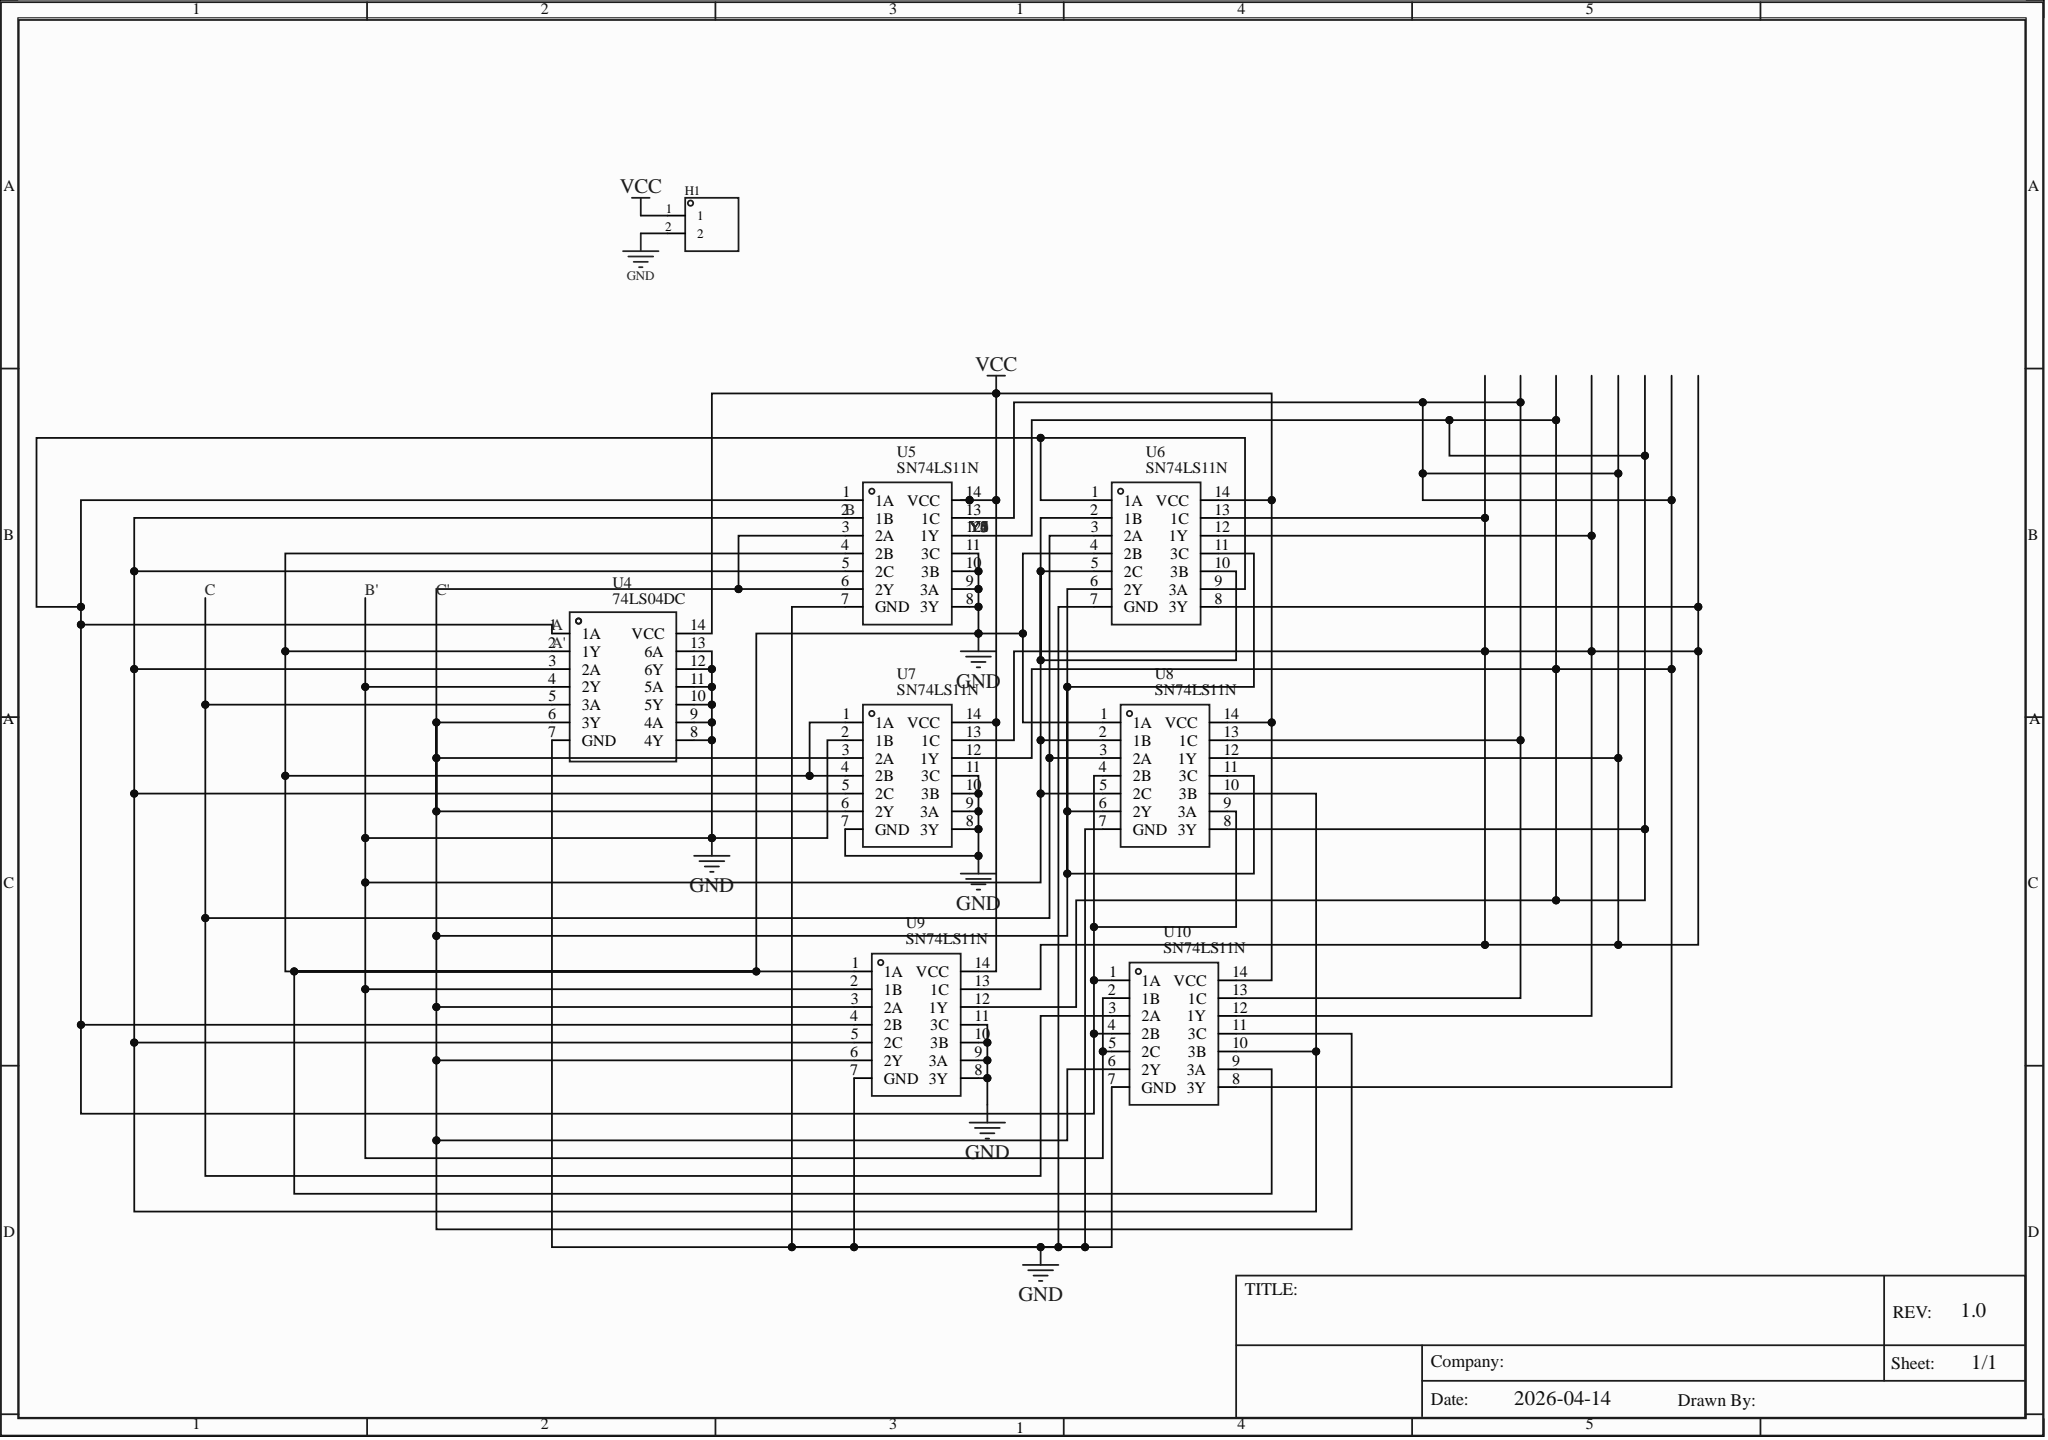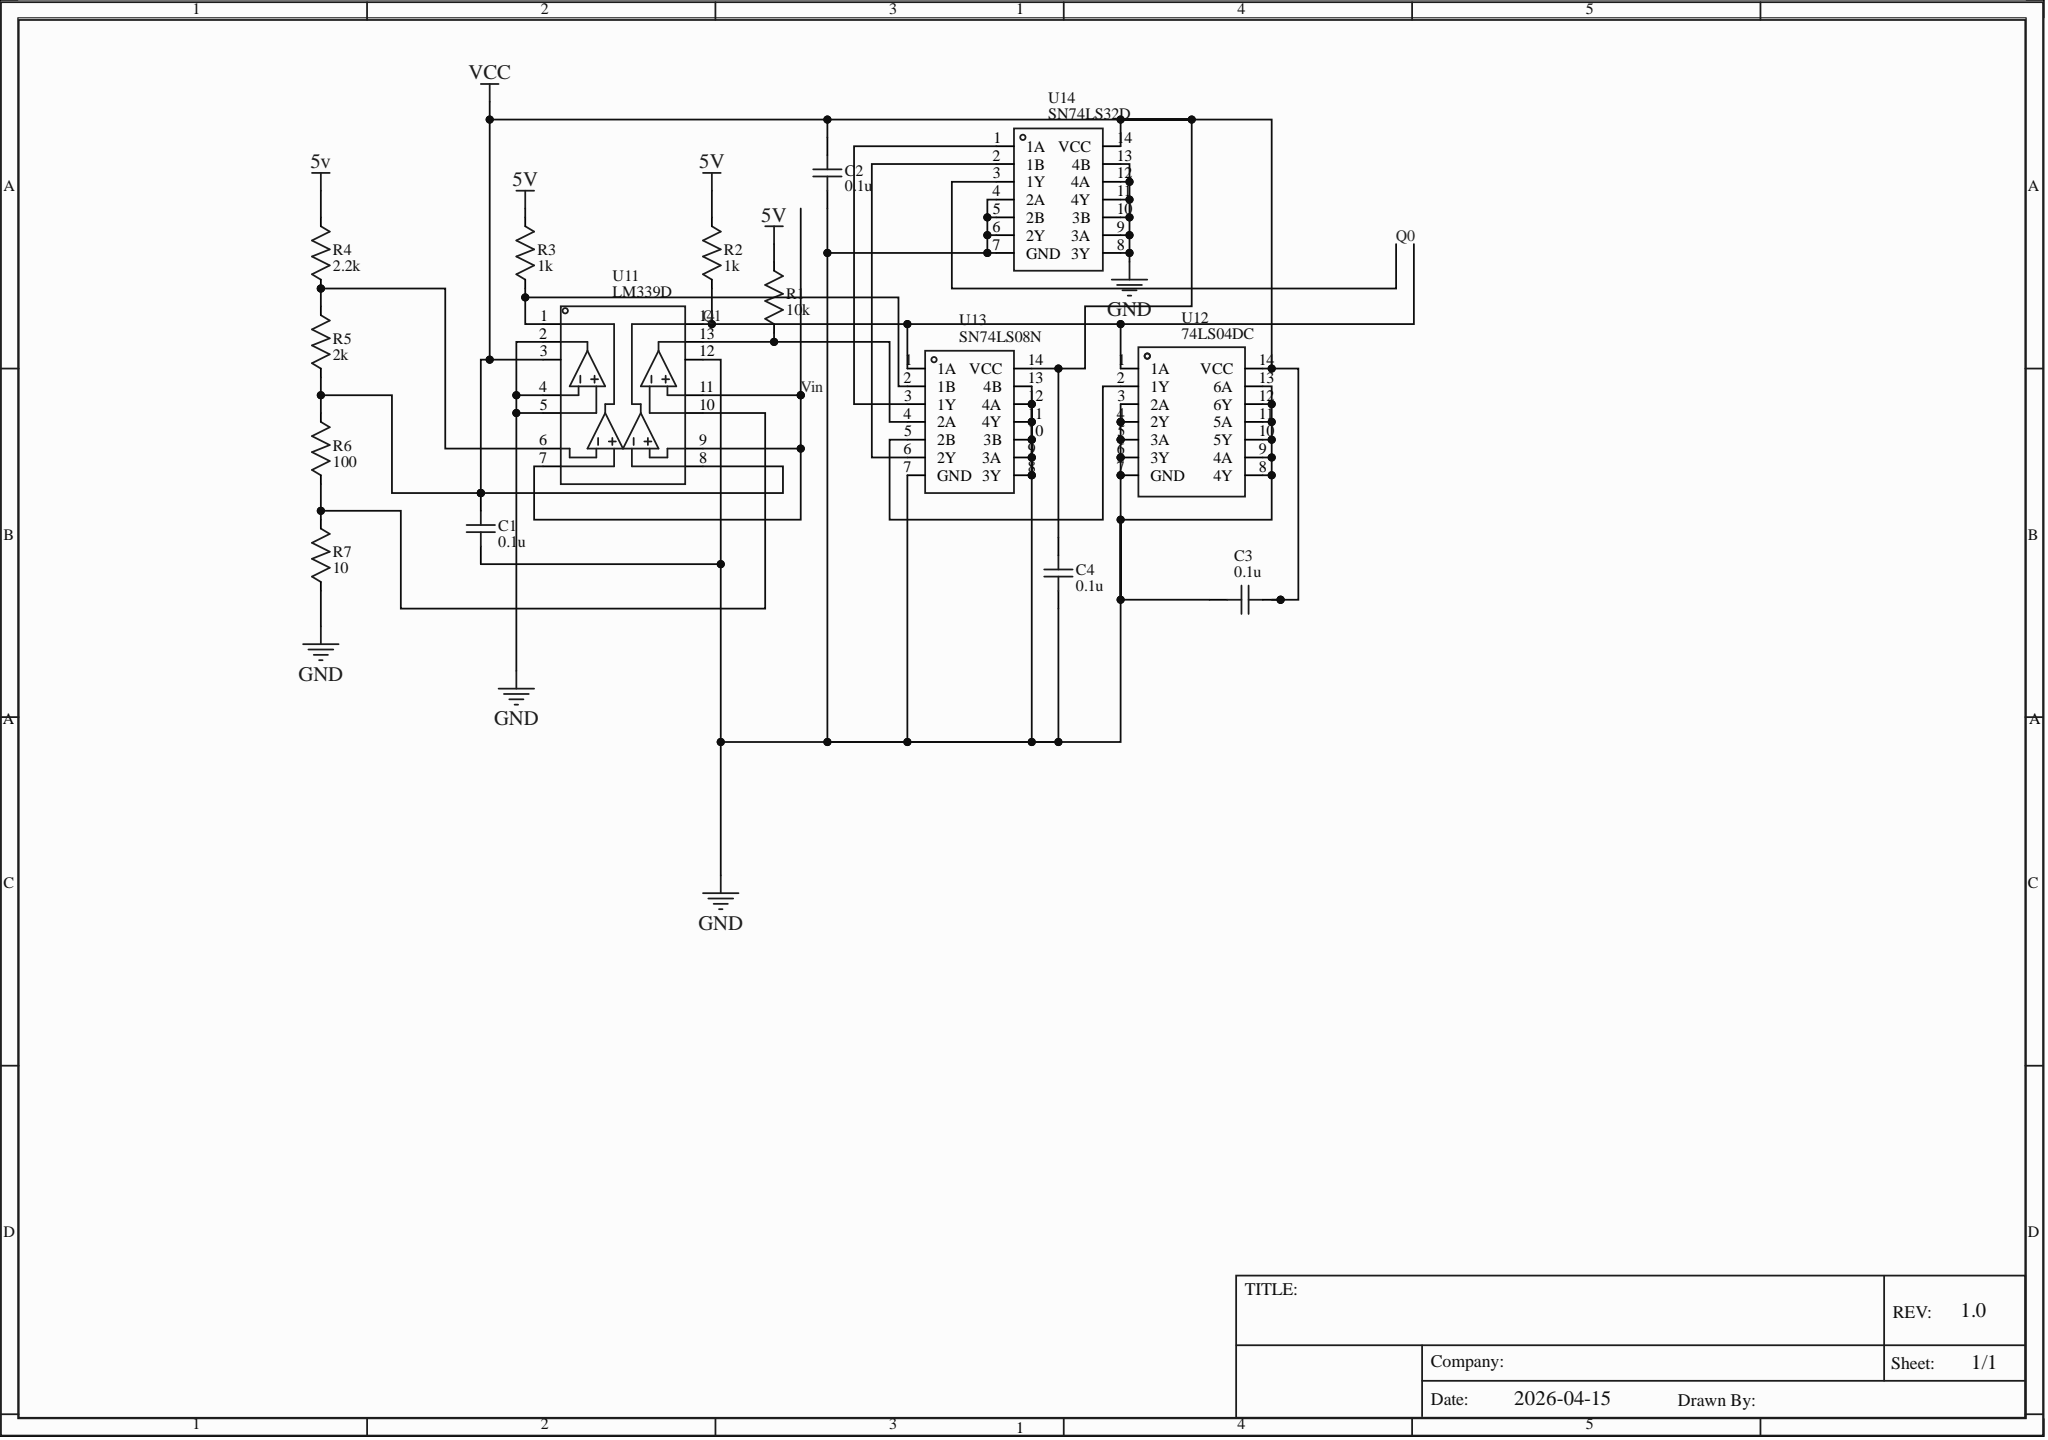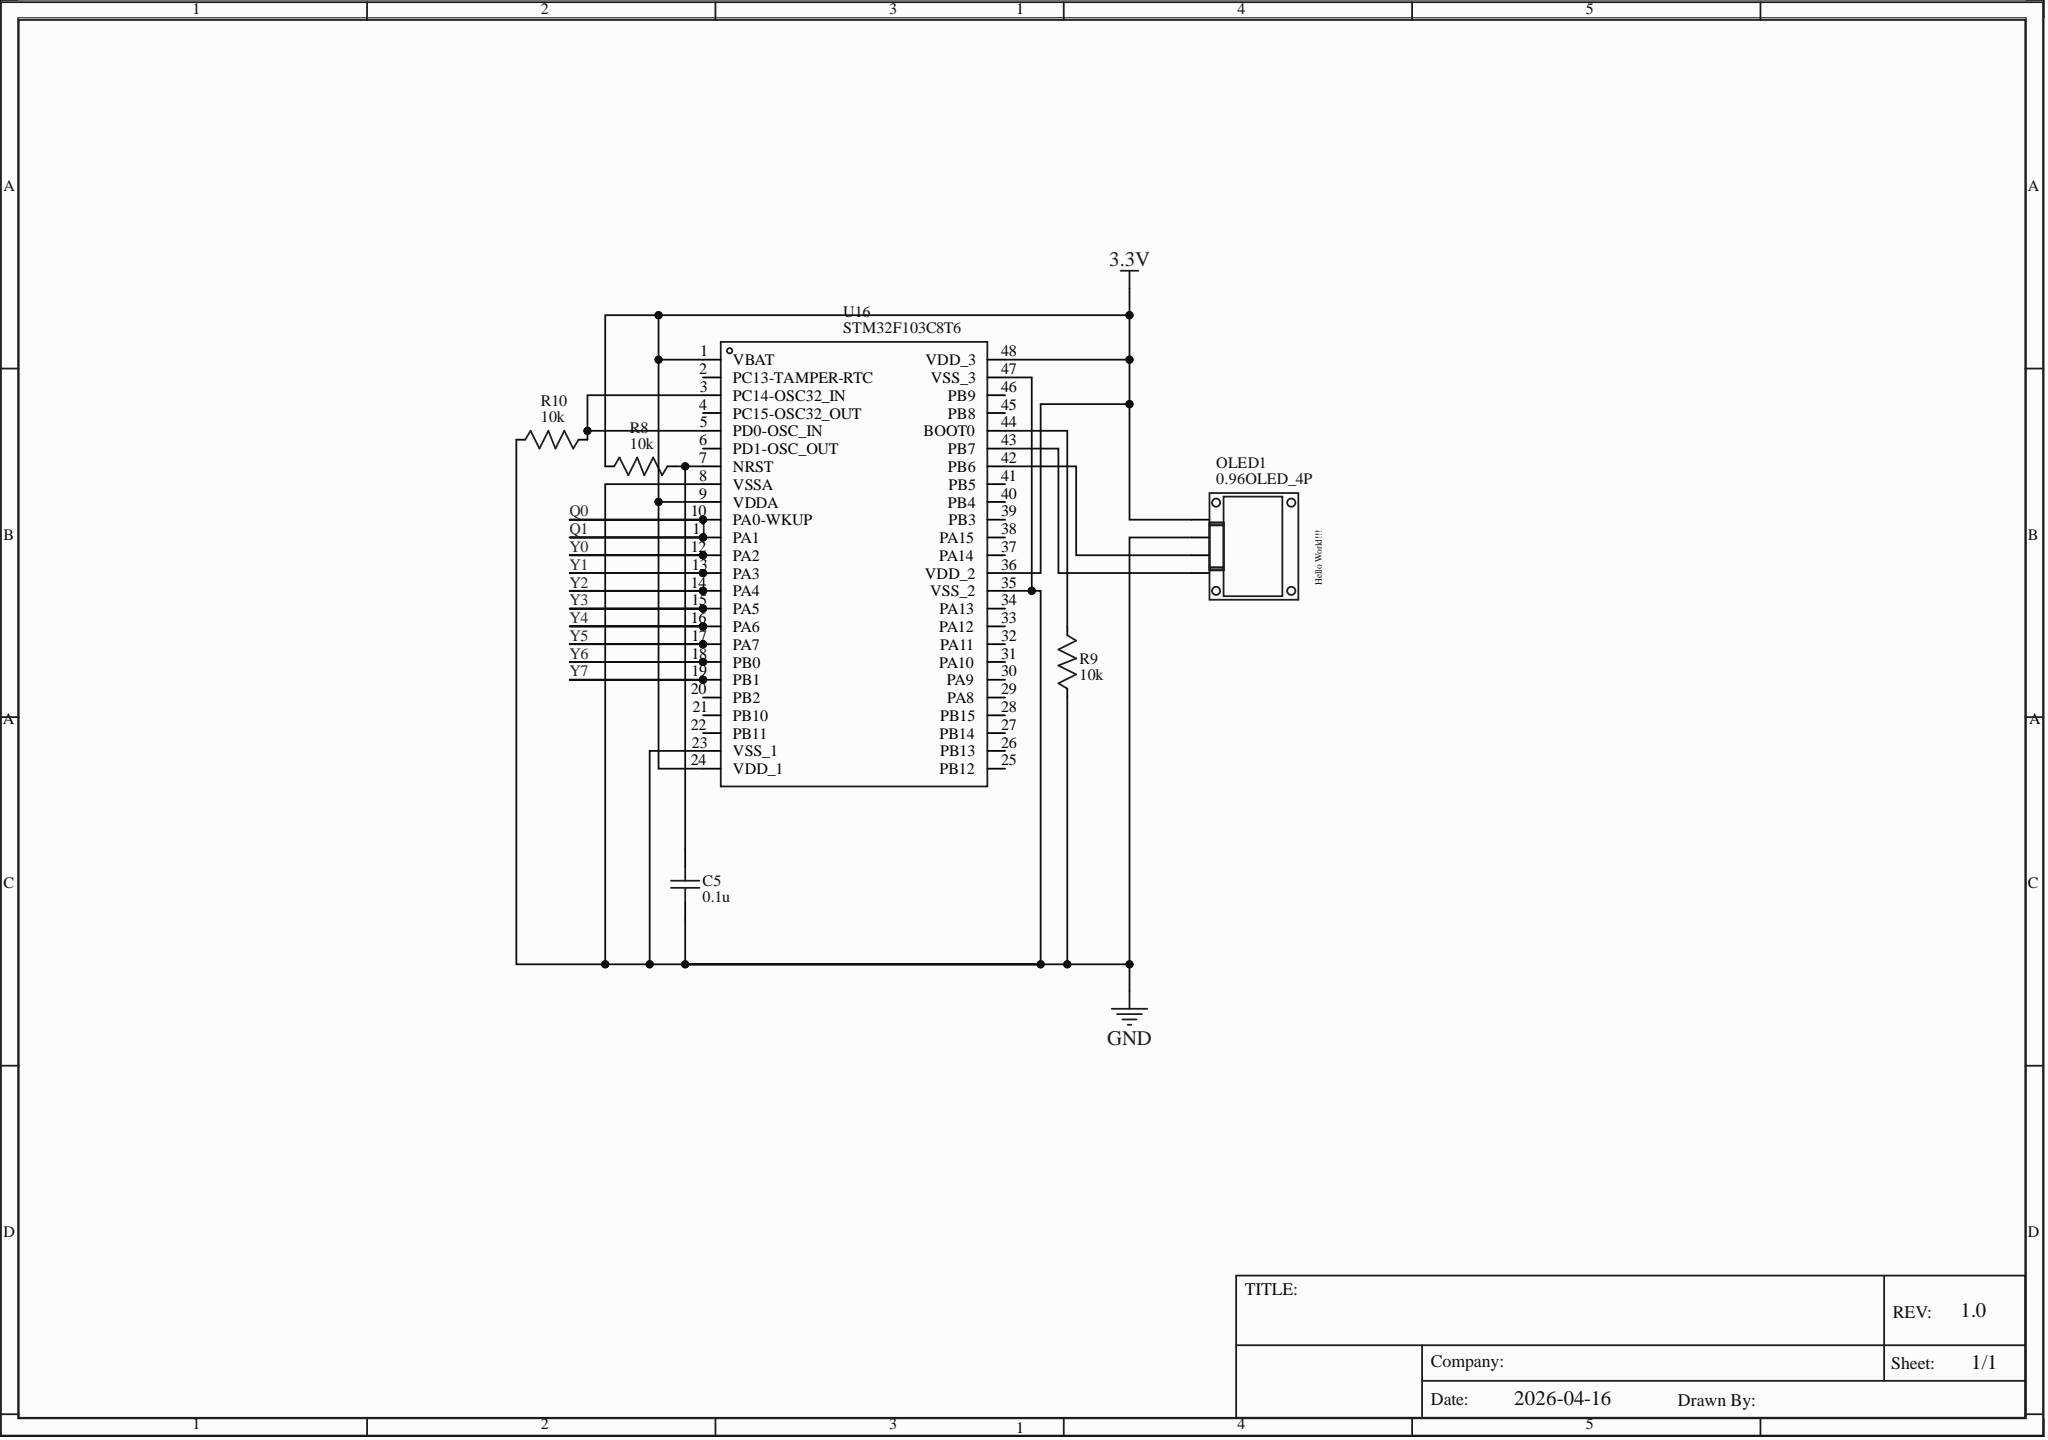Circuit board | Altium Designer | 29 parts | 24 nets
Bill of materials:
Comment,Description,Designator,Footprint,LibRef,Quantity
"0.1u","","C1, C2, C3, C4, C5","C0603","0.1u","5"
"","","H1","HDR-TH_2P-P2.54-V-M-1","HDR-M_2.54_1x2P","1"
"0.96OLED_4P","","OLED1","0.96OLED_4P","0.96OLED_4P","1"
"10k","","R1, R8, R9, R10","R0603","10k","4"
"1k","","R2, R3","R0603","1k","2"
"2.2k","","R4","R0603","2.2k","1"
"2k","","R5","R0603","2k","1"
"100","","R6","R0603","100","1"
"10","","R7","R0603","10","1"
"74LS04DC","","U4, U12","CDIP-14_L20.0-W6.8-P2.54-LS7.8-BL","74LS04DC","2"
"SN74LS11N","","U5, U6, U7, U8, U9, U10","PDIP-14_L19.3-W6.4-P2.54-LS7.9-BL-1","SN74LS11N","6"
"LM339D","","U11","SOIC-14_L8.7-W3.9-P1.27-LS6.0-BL","LM339D","1"
"SN74LS08N","","U13","PDIP-14_L19.3-W6.4-P2.54-LS7.9-BL-1","SN74LS08N","1"
"SN74LS32D","","U14","SOIC-14_L8.7-W3.9-P1.27-LS6.0-BL","SN74LS32D","1"
"STM32F103C8T6","","U16","LQFP-48_L7.0-W7.0-P0.50-LS9.0-BL","STM32F103C8T6","1"
Netlist (Protel format):
[
C1
C0603
0.1u



]
[
C2
C0603
0.1u



]
[
C3
C0603
0.1u



]
[
C4
C0603
0.1u



]
[
C5
C0603
0.1u



]
[
H1
HDR-TH_2P-P2.54-V-M-1




]
[
OLED1
0.96OLED_4P
0.96OLED_4P



]
[
R1
R0603
10k



]
[
R2
R0603
1k



]
[
R3
R0603
1k



]
[
R4
R0603
2.2k



]
[
R5
R0603
2k



]
[
R6
R0603
100



]
[
R7
R0603
10



]
[
R8
R0603
10k



]
[
R9
R0603
10k



]
[
R10
R0603
10k



]
[
U4
CDIP-14_L20.0-W6.8-P2.54-LS7.8-BL
74LS04DC



]
[
U5
PDIP-14_L19.3-W6.4-P2.54-LS7.9-BL-1
SN74LS11N



]
[
U6
PDIP-14_L19.3-W6.4-P2.54-LS7.9-BL-1
SN74LS11N



]
[
U7
PDIP-14_L19.3-W6.4-P2.54-LS7.9-BL-1
SN74LS11N



]
[
U8
PDIP-14_L19.3-W6.4-P2.54-LS7.9-BL-1
SN74LS11N



]
[
U9
PDIP-14_L19.3-W6.4-P2.54-LS7.9-BL-1
SN74LS11N



]
[
U10
PDIP-14_L19.3-W6.4-P2.54-LS7.9-BL-1
SN74LS11N



]
[
U11
SOIC-14_L8.7-W3.9-P1.27-LS6.0-BL
LM339D



]
[
U12
CDIP-14_L20.0-W6.8-P2.54-LS7.8-BL
74LS04DC



]
[
U13
PDIP-14_L19.3-W6.4-P2.54-LS7.9-BL-1
SN74LS08N



]
[
U14
SOIC-14_L8.7-W3.9-P1.27-LS6.0-BL
SN74LS32D



]
[
U16
LQFP-48_L7.0-W7.0-P0.50-LS9.0-BL
STM32F103C8T6



]
(
Y0
U5-12
U5-13
U6-8
U6-12
U6-13
U7-12
U7-13
U8-8
U8-12
U8-13
U9-12
U9-13
U10-8
U10-12
U10-13
U16-12
U16-13
U16-14
U16-15
U16-16
U16-17
U16-18
U16-19
)
(
Vin
U11-7
U11-9
U11-11
)
(
VCC
C1-2
C2-2
C3-2
C4-2
H1-1
R5-1
R6-2
U4-14
U5-14
U6-14
U7-14
U8-14
U9-14
U10-14
U11-3
U11-8
U12-14
U13-14
U14-14
)
(
Q1
R2-1
U11-14
U12-1
U13-1
U16-11
)
(
Q0
U14-3
U16-10
)
(
NetU13_6
U13-6
U14-2
)
(
NetU13_3
U13-3
U14-1
)
(
NetU12_2
U12-2
U13-5
)
(
NetR10_2
R10-2
U16-3
U16-5
)
(
NetR9_2
R9-2
U16-44
)
(
NetR6_1
R6-1
R7-2
U11-10
)
(
NetR4_1
R4-1
R5-2
U11-6
)
(
NetR3_1
R3-1
U11-1
U13-2
)
(
NetR1_2
R1-2
U11-13
U13-4
)
(
NetOLED1_4
OLED1-4
U16-43
)
(
NetOLED1_3
OLED1-3
U16-42
)
(
NetC5_2
C5-2
R8-2
U16-7
)
(
C'
U4-6
U5-3
U5-6
U6-6
U6-11
U7-3
U7-6
U8-6
U8-11
U9-3
U9-6
U10-6
U10-11
)
(
C
U4-5
U6-3
U8-3
U10-3
)
(
B
U4-3
U5-2
U5-5
U7-5
U8-10
U9-5
U10-10
)
(
A'
C1-1
C2-1
C3-1
C4-1
C5-1
H1-2
OLED1-2
R7-1
R9-1
R10-1
U4-2
U4-4
U4-7
U4-8
U4-9
U4-10
U4-11
U4-12
U4-13
U5-4
U5-7
U5-8
U5-9
U5-10
U5-11
U6-2
U6-4
U6-5
U6-7
U6-10
U7-1
U7-2
U7-4
U7-7
U7-8
U7-9
U7-10
U7-11
U8-1
U8-2
U8-5
U8-7
U9-1
U9-2
U9-7
U9-8
U9-9
U9-10
U9-11
U10-2
U10-5
U10-7
U10-9
U11-2
U11-4
U11-5
U11-12
U12-3
U12-4
U12-5
U12-6
U12-7
U12-8
U12-9
U12-10
U12-11
U12-12
U12-13
U13-7
U13-8
U13-9
U13-10
U13-11
U13-12
U13-13
U14-4
U14-5
U14-6
U14-7
U14-8
U14-9
U14-10
U14-11
U14-12
U14-13
U16-8
U16-23
U16-35
U16-47
)
(
A
U4-1
U5-1
U6-1
U6-9
U8-4
U8-9
U9-4
U10-1
U10-4
)
(
5v
R1-1
R2-2
R3-2
R4-2
)
(
3.3V
OLED1-1
R8-1
U16-1
U16-9
U16-24
U16-36
U16-48
)